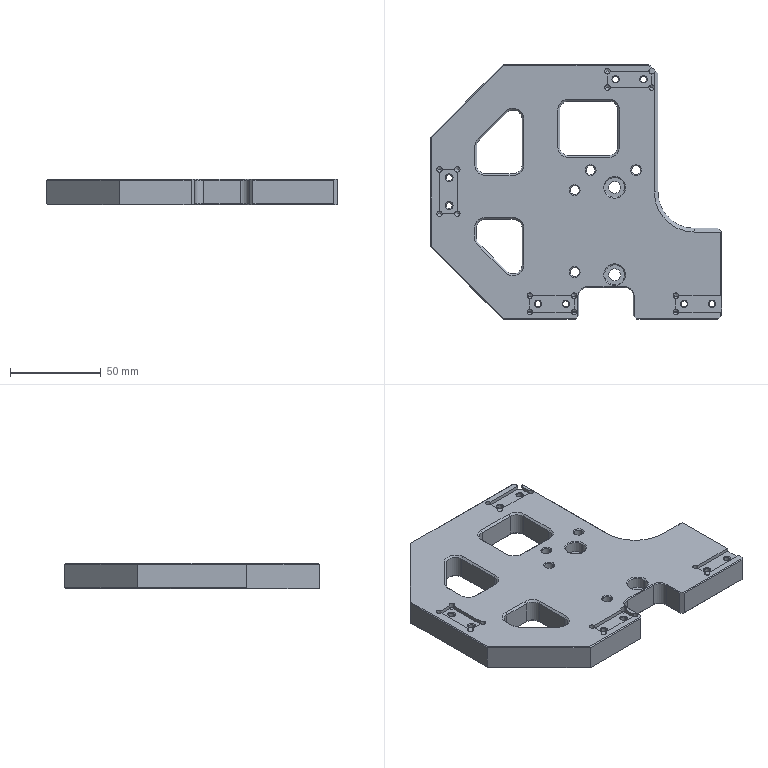Part | SolidWorks | features MoveFace 6, ICE 2, Chamfer 1, DelFace 1, HoleWzd 1, MirrorStock 1 | 1 solid | 272 faces | box 160 x 140 x 14 mm | volume 203206 mm3 | plane 105 | cone 92 | cylinder 75 | commonest cylinder face diameters 3 x28 3.3 x16 10 x14 5 x8 6.5 x4 11 x4